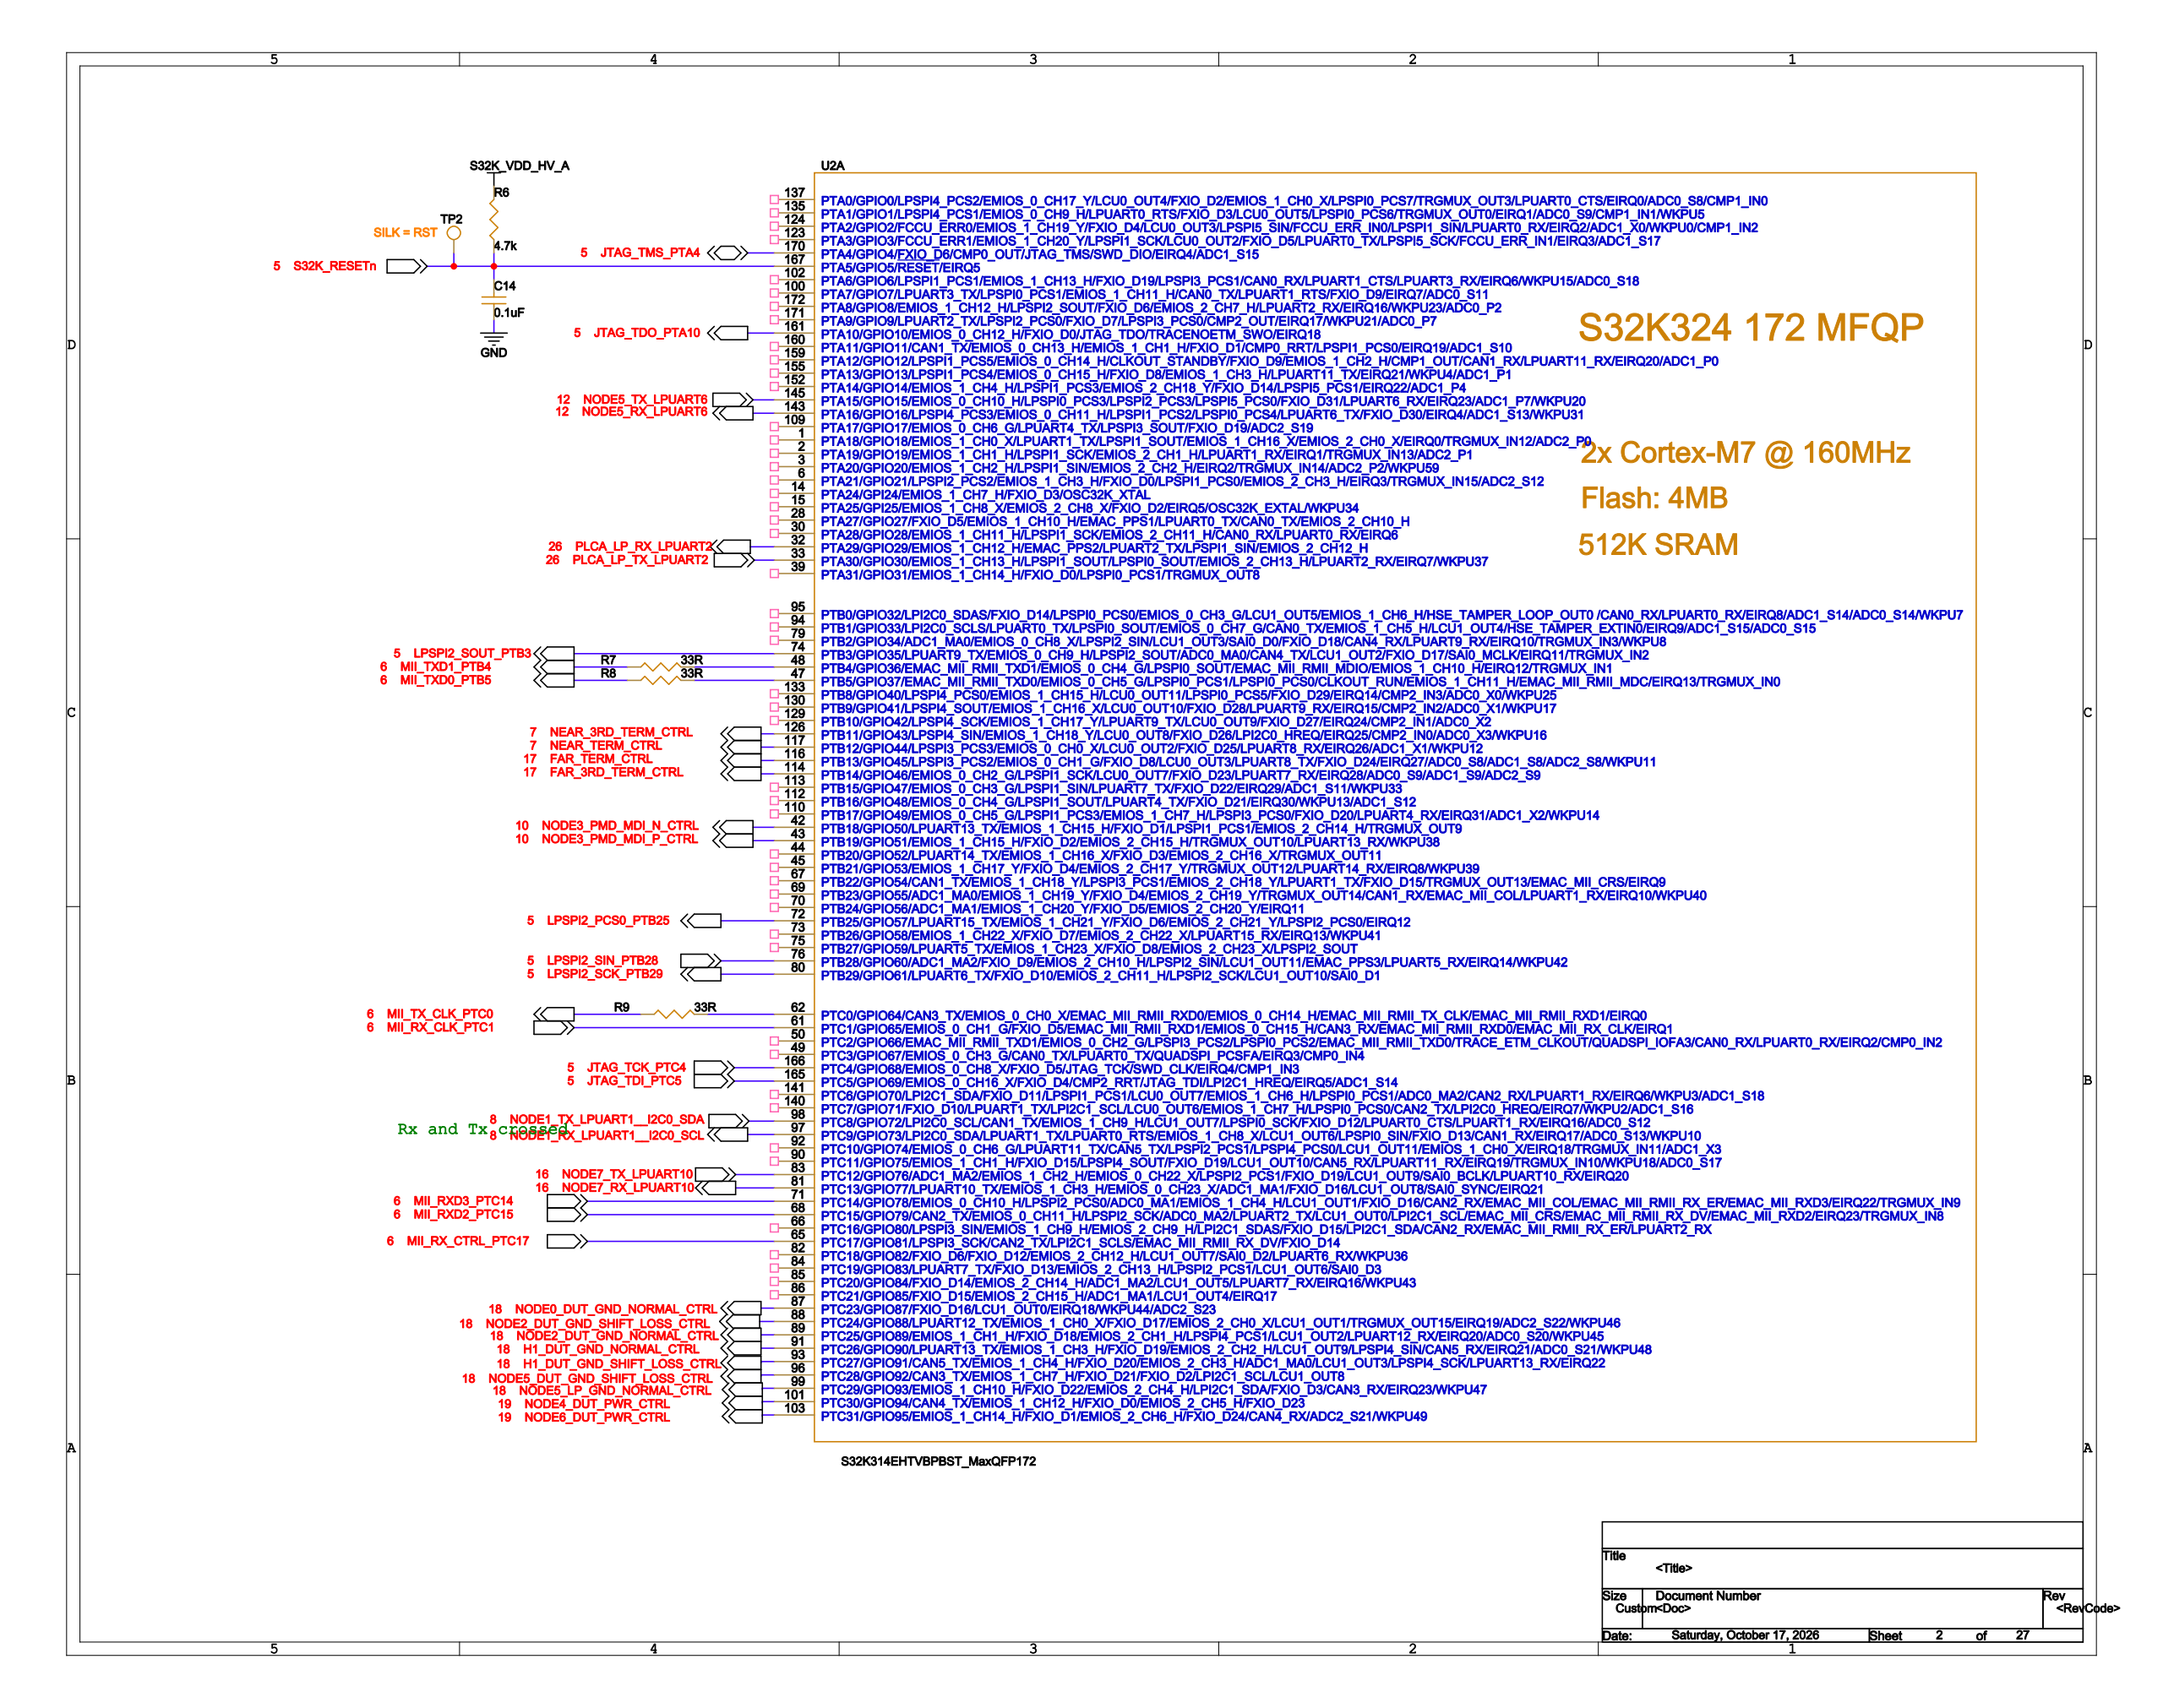Circuit board | Cadence Allegro | 477 parts | 327 nets | one sheet of the schematic
Parts on this sheet (reference | value | footprint):
C14 | 0.1uF | 0402
R6 | 4.7K | 0402
R7 | 33R | 0402
R8 | 33R | 0402
R9 | 33R | 0402
TP2 | TP | S0400CI
U2 | S32K314EHTVBPBST_MaxQFP172 | MQFP172_0P65_16X16
Nets of these parts (net: part-pin ...):
JTAG_TCK_PTC4: U2-166
JTAG_TDO_PTA10: U2-161
JTAG_TMS_PTA4: U2-170
JTAG_TDI_PTC5: U2-165
MII_RX_CLK_PTC1: U2-61
MII_RXD2_PTC15: U2-68
MII_RXD3_PTC14: U2-71
MII_RX_CTRL_PTC17: U2-65
MII_TXD1_PTB4: R7-1
N2514309: R7-2 U2-48
MII_TXD0_PTB5: R8-1
N2514313: R8-2 U2-47
MII_TX_CLK_PTC0: R9-1
N2514360: R9-2 U2-62
NODE5_LP_GND_NORMAL_CTRL: U2-99
NODE5_DUT_GND_SHIFT_LOSS_CTRL: U2-96
NODE4_DUT_PWR_CTRL: U2-101
NODE3_PMD_MDI_N_CTRL: U2-42
NODE3_PMD_MDI_P_CTRL: U2-43
GND: C14-1 U2-17
S32K_VDD_HV_A: R6-1 U2-16 U2-18
LPSPI2_PCS0_PTB25: U2-72
S32K_RESETN: C14-2 R6-2 TP2-1 U2-167
NODE5_TX_LPUART6: U2-145
NODE5_RX_LPUART6: U2-143
NODE7_TX_LPUART10: U2-83
NODE7_RX_LPUART10: U2-81
PLCA_LP_TX_LPUART2: U2-33
PLCA_LP_RX_LPUART2: U2-32
NODE1_TX_LPUART1__I2C0_SDA: U2-98
NODE1_RX_LPUART1__I2C0_SCL: U2-97
NEAR_3RD_TERM_CTRL: U2-126
NEAR_TERM_CTRL: U2-117
FAR_TERM_CTRL: U2-116
FAR_3RD_TERM_CTRL: U2-114
LPSPI2_SIN_PTB28: U2-76
LPSPI2_SCK_PTB29: U2-80
LPSPI2_SOUT_PTB3: U2-74
NODE0_DUT_GND_NORMAL_CTRL: U2-87
NODE2_DUT_GND_SHIFT_LOSS_CTRL: U2-88
NODE2_DUT_GND_NORMAL_CTRL: U2-89
H1_DUT_GND_NORMAL_CTRL: U2-91
H1_DUT_GND_SHIFT_LOSS_CTRL: U2-93
NODE6_DUT_PWR_CTRL: U2-103